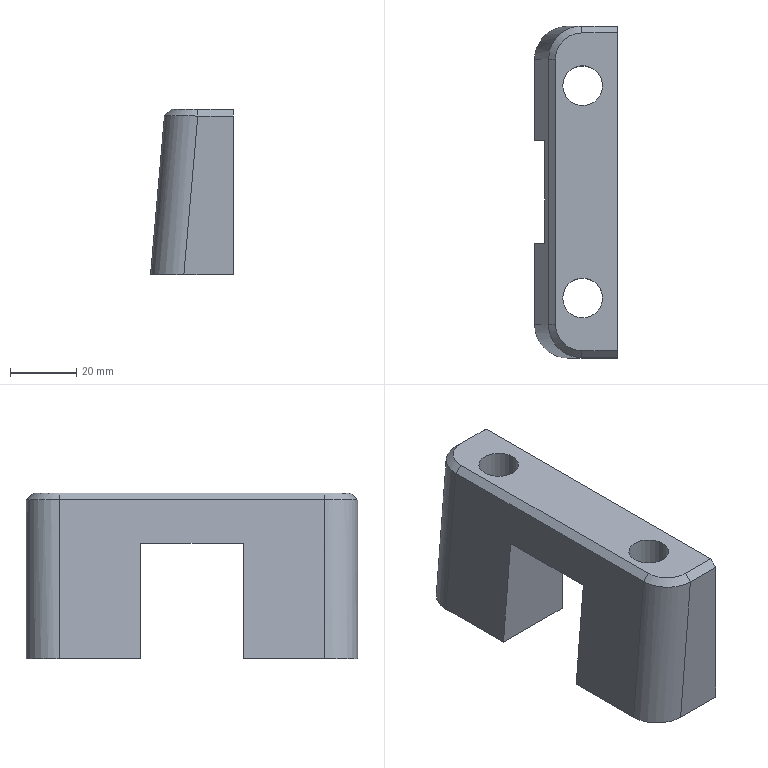Part | STEP file | solid 73 | 1 solid | 23 faces | box 25 x 100 x 50 mm | volume 71531 mm3 | plane 15 | cylinder 6 | spline 2 | commonest cylinder face diameters 12 x2 18 x2 20 x2